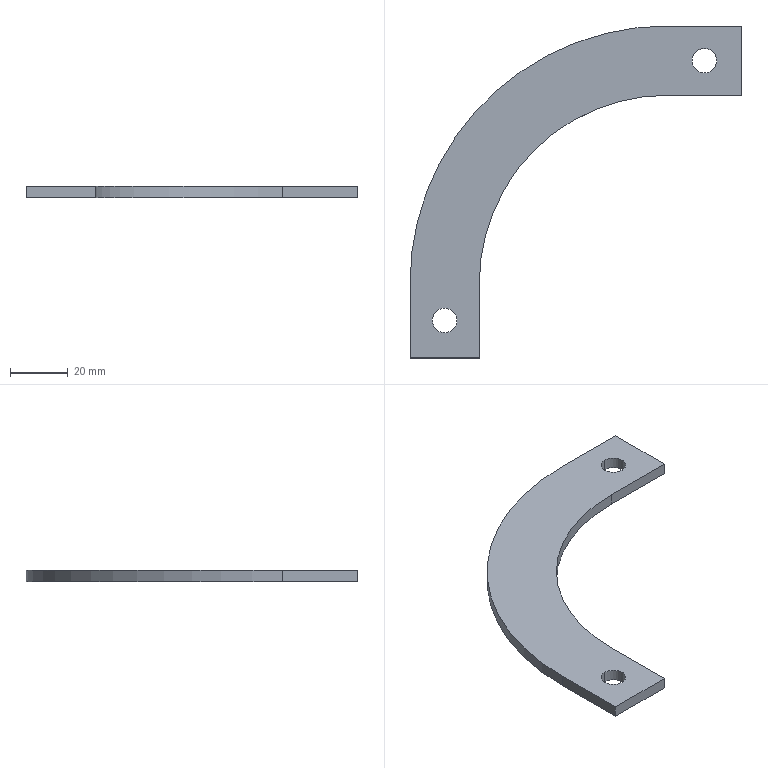Part | SolidWorks | features BaseBody 1 | 1 solid | 14 faces | box 115 x 115 x 4 mm | volume 16149 mm3 | plane 8 | cylinder 6 | commonest cylinder face diameters 8.5 x4 130 x1 178 x1
STEP:
#1=CARTESIAN_POINT('',(273.,59.25,281.));
#2=VERTEX_POINT('',#1);
#3=CARTESIAN_POINT('',(273.,50.75,281.));
#4=VERTEX_POINT('',#3);
#5=CARTESIAN_POINT('',(273.,55.,281.));
#6=DIRECTION('',(0.,0.,1.));
#7=DIRECTION('',(0.,1.,0.));
#8=AXIS2_PLACEMENT_3D('',#5,#6,#7);
#9=CIRCLE('',#8,4.25);
#10=EDGE_CURVE('',#2,#4,#9,.T.);
#11=ORIENTED_EDGE('',*,*,#10,.T.);
#12=CARTESIAN_POINT('',(273.,50.75,277.));
#13=VERTEX_POINT('',#12);
#14=CARTESIAN_POINT('',(273.,50.75,281.));
#15=DIRECTION('',(0.,0.,-1.));
#16=VECTOR('',#15,1000.);
#17=LINE('',#14,#16);
#18=EDGE_CURVE('',#4,#13,#17,.T.);
#19=ORIENTED_EDGE('',*,*,#18,.T.);
#20=CARTESIAN_POINT('',(273.,59.25,277.));
#21=VERTEX_POINT('',#20);
#22=CARTESIAN_POINT('',(273.,55.,277.));
#23=DIRECTION('',(0.,0.,-1.));
#24=DIRECTION('',(0.,-1.,0.));
#25=AXIS2_PLACEMENT_3D('',#22,#23,#24);
#26=CIRCLE('',#25,4.25);
#27=EDGE_CURVE('',#13,#21,#26,.T.);
#28=ORIENTED_EDGE('',*,*,#27,.T.);
#29=CARTESIAN_POINT('',(273.,59.25,281.));
#30=DIRECTION('',(0.,0.,-1.));
#31=VECTOR('',#30,1000.);
#32=LINE('',#29,#31);
#33=EDGE_CURVE('',#2,#21,#32,.T.);
#34=ORIENTED_EDGE('',*,*,#33,.F.);
#35=EDGE_LOOP('',(#11,#19,#28,#34));
#36=FACE_OUTER_BOUND('',#35,.T.);
#37=CARTESIAN_POINT('',(273.,55.,281.));
#38=DIRECTION('',(0.,0.,-1.));
#39=DIRECTION('',(0.,1.,0.));
#40=AXIS2_PLACEMENT_3D('',#37,#38,#39);
#41=CYLINDRICAL_SURFACE('',#40,4.25);
#42=ADVANCED_FACE('',(#36),#41,.F.);
#43=CARTESIAN_POINT('',(183.,-30.75,281.));
#44=VERTEX_POINT('',#43);
#45=CARTESIAN_POINT('',(183.,-39.25,281.));
#46=VERTEX_POINT('',#45);
#47=CARTESIAN_POINT('',(183.,-35.,281.));
#48=DIRECTION('',(0.,0.,1.));
#49=DIRECTION('',(0.,1.,0.));
#50=AXIS2_PLACEMENT_3D('',#47,#48,#49);
#51=CIRCLE('',#50,4.25);
#52=EDGE_CURVE('',#44,#46,#51,.T.);
#53=ORIENTED_EDGE('',*,*,#52,.T.);
#54=CARTESIAN_POINT('',(183.,-39.25,277.));
#55=VERTEX_POINT('',#54);
#56=CARTESIAN_POINT('',(183.,-39.25,281.));
#57=DIRECTION('',(0.,0.,-1.));
#58=VECTOR('',#57,1000.);
#59=LINE('',#56,#58);
#60=EDGE_CURVE('',#46,#55,#59,.T.);
#61=ORIENTED_EDGE('',*,*,#60,.T.);
#62=CARTESIAN_POINT('',(183.,-30.75,277.));
#63=VERTEX_POINT('',#62);
#64=CARTESIAN_POINT('',(183.,-35.,277.));
#65=DIRECTION('',(0.,0.,-1.));
#66=DIRECTION('',(0.,-1.,0.));
#67=AXIS2_PLACEMENT_3D('',#64,#65,#66);
#68=CIRCLE('',#67,4.25);
#69=EDGE_CURVE('',#55,#63,#68,.T.);
#70=ORIENTED_EDGE('',*,*,#69,.T.);
#71=CARTESIAN_POINT('',(183.,-30.75,281.));
#72=DIRECTION('',(0.,0.,-1.));
#73=VECTOR('',#72,1000.);
#74=LINE('',#71,#73);
#75=EDGE_CURVE('',#44,#63,#74,.T.);
#76=ORIENTED_EDGE('',*,*,#75,.F.);
#77=EDGE_LOOP('',(#53,#61,#70,#76));
#78=FACE_OUTER_BOUND('',#77,.T.);
#79=CARTESIAN_POINT('',(183.,-35.,281.));
#80=DIRECTION('',(0.,0.,-1.));
#81=DIRECTION('',(0.,1.,0.));
#82=AXIS2_PLACEMENT_3D('',#79,#80,#81);
#83=CYLINDRICAL_SURFACE('',#82,4.25);
#84=ADVANCED_FACE('',(#78),#83,.F.);
#85=CARTESIAN_POINT('',(183.,-35.,277.));
#86=DIRECTION('',(0.,0.,-1.));
#87=DIRECTION('',(0.,-1.,0.));
#88=AXIS2_PLACEMENT_3D('',#85,#86,#87);
#89=CIRCLE('',#88,4.25);
#90=EDGE_CURVE('',#63,#55,#89,.T.);
#91=ORIENTED_EDGE('',*,*,#90,.F.);
#92=ORIENTED_EDGE('',*,*,#69,.F.);
#93=EDGE_LOOP('',(#91,#92));
#94=FACE_BOUND('',#93,.T.);
#95=CARTESIAN_POINT('',(273.,55.,277.));
#96=DIRECTION('',(0.,0.,-1.));
#97=DIRECTION('',(0.,-1.,0.));
#98=AXIS2_PLACEMENT_3D('',#95,#96,#97);
#99=CIRCLE('',#98,4.25);
#100=EDGE_CURVE('',#21,#13,#99,.T.);
#101=ORIENTED_EDGE('',*,*,#100,.F.);
#102=ORIENTED_EDGE('',*,*,#27,.F.);
#103=EDGE_LOOP('',(#101,#102));
#104=FACE_BOUND('',#103,.T.);
#105=CARTESIAN_POINT('',(171.,-22.,277.));
#106=VERTEX_POINT('',#105);
#107=CARTESIAN_POINT('',(171.,-48.,277.));
#108=VERTEX_POINT('',#107);
#109=CARTESIAN_POINT('',(171.,-22.,277.));
#110=DIRECTION('',(0.,-1.,0.));
#111=VECTOR('',#110,1000.);
#112=LINE('',#109,#111);
#113=EDGE_CURVE('',#106,#108,#112,.T.);
#114=ORIENTED_EDGE('',*,*,#113,.F.);
#115=CARTESIAN_POINT('',(260.,67.,277.));
#116=VERTEX_POINT('',#115);
#117=CARTESIAN_POINT('',(260.,-22.,277.));
#118=DIRECTION('',(0.,0.,1.));
#119=DIRECTION('',(0.,1.,0.));
#120=AXIS2_PLACEMENT_3D('',#117,#118,#119);
#121=CIRCLE('',#120,89.);
#122=EDGE_CURVE('',#116,#106,#121,.T.);
#123=ORIENTED_EDGE('',*,*,#122,.F.);
#124=CARTESIAN_POINT('',(286.,67.,277.));
#125=VERTEX_POINT('',#124);
#126=CARTESIAN_POINT('',(286.,67.,277.));
#127=DIRECTION('',(-1.,0.,0.));
#128=VECTOR('',#127,1000.);
#129=LINE('',#126,#128);
#130=EDGE_CURVE('',#125,#116,#129,.T.);
#131=ORIENTED_EDGE('',*,*,#130,.F.);
#132=CARTESIAN_POINT('',(286.,43.,277.));
#133=VERTEX_POINT('',#132);
#134=CARTESIAN_POINT('',(286.,43.,277.));
#135=DIRECTION('',(0.,1.,0.));
#136=VECTOR('',#135,1000.);
#137=LINE('',#134,#136);
#138=EDGE_CURVE('',#133,#125,#137,.T.);
#139=ORIENTED_EDGE('',*,*,#138,.F.);
#140=CARTESIAN_POINT('',(260.,43.,277.));
#141=VERTEX_POINT('',#140);
#142=CARTESIAN_POINT('',(260.,43.,277.));
#143=DIRECTION('',(1.,0.,0.));
#144=VECTOR('',#143,1000.);
#145=LINE('',#142,#144);
#146=EDGE_CURVE('',#141,#133,#145,.T.);
#147=ORIENTED_EDGE('',*,*,#146,.F.);
#148=CARTESIAN_POINT('',(195.,-22.,277.));
#149=VERTEX_POINT('',#148);
#150=CARTESIAN_POINT('',(260.,-22.,277.));
#151=DIRECTION('',(0.,0.,-1.));
#152=DIRECTION('',(-1.,0.,0.));
#153=AXIS2_PLACEMENT_3D('',#150,#151,#152);
#154=CIRCLE('',#153,65.);
#155=EDGE_CURVE('',#149,#141,#154,.T.);
#156=ORIENTED_EDGE('',*,*,#155,.F.);
#157=CARTESIAN_POINT('',(195.,-48.,277.));
#158=VERTEX_POINT('',#157);
#159=CARTESIAN_POINT('',(195.,-48.,277.));
#160=DIRECTION('',(0.,1.,0.));
#161=VECTOR('',#160,1000.);
#162=LINE('',#159,#161);
#163=EDGE_CURVE('',#158,#149,#162,.T.);
#164=ORIENTED_EDGE('',*,*,#163,.F.);
#165=CARTESIAN_POINT('',(171.,-48.,277.));
#166=DIRECTION('',(1.,0.,0.));
#167=VECTOR('',#166,1000.);
#168=LINE('',#165,#167);
#169=EDGE_CURVE('',#108,#158,#168,.T.);
#170=ORIENTED_EDGE('',*,*,#169,.F.);
#171=EDGE_LOOP('',(#114,#123,#131,#139,#147,#156,#164,#170));
#172=FACE_OUTER_BOUND('',#171,.T.);
#173=CARTESIAN_POINT('',(260.,-22.,277.));
#174=DIRECTION('',(0.,0.,-1.));
#175=DIRECTION('',(-1.,0.,0.));
#176=AXIS2_PLACEMENT_3D('',#173,#174,#175);
#177=PLANE('',#176);
#178=ADVANCED_FACE('',(#94,#104,#172),#177,.T.);
#179=ORIENTED_EDGE('',*,*,#52,.F.);
#180=CARTESIAN_POINT('',(183.,-35.,281.));
#181=DIRECTION('',(0.,0.,1.));
#182=DIRECTION('',(0.,1.,0.));
#183=AXIS2_PLACEMENT_3D('',#180,#181,#182);
#184=CIRCLE('',#183,4.25);
#185=EDGE_CURVE('',#46,#44,#184,.T.);
#186=ORIENTED_EDGE('',*,*,#185,.F.);
#187=EDGE_LOOP('',(#179,#186));
#188=FACE_BOUND('',#187,.T.);
#189=ORIENTED_EDGE('',*,*,#10,.F.);
#190=CARTESIAN_POINT('',(273.,55.,281.));
#191=DIRECTION('',(0.,0.,1.));
#192=DIRECTION('',(0.,1.,0.));
#193=AXIS2_PLACEMENT_3D('',#190,#191,#192);
#194=CIRCLE('',#193,4.25);
#195=EDGE_CURVE('',#4,#2,#194,.T.);
#196=ORIENTED_EDGE('',*,*,#195,.F.);
#197=EDGE_LOOP('',(#189,#196));
#198=FACE_BOUND('',#197,.T.);
#199=CARTESIAN_POINT('',(171.,-48.,281.));
#200=VERTEX_POINT('',#199);
#201=CARTESIAN_POINT('',(171.,-22.,281.));
#202=VERTEX_POINT('',#201);
#203=CARTESIAN_POINT('',(171.,-48.,281.));
#204=DIRECTION('',(0.,1.,0.));
#205=VECTOR('',#204,1000.);
#206=LINE('',#203,#205);
#207=EDGE_CURVE('',#200,#202,#206,.T.);
#208=ORIENTED_EDGE('',*,*,#207,.F.);
#209=CARTESIAN_POINT('',(195.,-48.,281.));
#210=VERTEX_POINT('',#209);
#211=CARTESIAN_POINT('',(195.,-48.,281.));
#212=DIRECTION('',(-1.,0.,0.));
#213=VECTOR('',#212,1000.);
#214=LINE('',#211,#213);
#215=EDGE_CURVE('',#210,#200,#214,.T.);
#216=ORIENTED_EDGE('',*,*,#215,.F.);
#217=CARTESIAN_POINT('',(195.,-22.,281.));
#218=VERTEX_POINT('',#217);
#219=CARTESIAN_POINT('',(195.,-22.,281.));
#220=DIRECTION('',(0.,-1.,0.));
#221=VECTOR('',#220,1000.);
#222=LINE('',#219,#221);
#223=EDGE_CURVE('',#218,#210,#222,.T.);
#224=ORIENTED_EDGE('',*,*,#223,.F.);
#225=CARTESIAN_POINT('',(260.,43.,281.));
#226=VERTEX_POINT('',#225);
#227=CARTESIAN_POINT('',(260.,-22.,281.));
#228=DIRECTION('',(0.,0.,1.));
#229=DIRECTION('',(0.,1.,0.));
#230=AXIS2_PLACEMENT_3D('',#227,#228,#229);
#231=CIRCLE('',#230,65.);
#232=EDGE_CURVE('',#226,#218,#231,.T.);
#233=ORIENTED_EDGE('',*,*,#232,.F.);
#234=CARTESIAN_POINT('',(286.,43.,281.));
#235=VERTEX_POINT('',#234);
#236=CARTESIAN_POINT('',(286.,43.,281.));
#237=DIRECTION('',(-1.,0.,0.));
#238=VECTOR('',#237,1000.);
#239=LINE('',#236,#238);
#240=EDGE_CURVE('',#235,#226,#239,.T.);
#241=ORIENTED_EDGE('',*,*,#240,.F.);
#242=CARTESIAN_POINT('',(286.,67.,281.));
#243=VERTEX_POINT('',#242);
#244=CARTESIAN_POINT('',(286.,67.,281.));
#245=DIRECTION('',(0.,-1.,0.));
#246=VECTOR('',#245,1000.);
#247=LINE('',#244,#246);
#248=EDGE_CURVE('',#243,#235,#247,.T.);
#249=ORIENTED_EDGE('',*,*,#248,.F.);
#250=CARTESIAN_POINT('',(260.,67.,281.));
#251=VERTEX_POINT('',#250);
#252=CARTESIAN_POINT('',(260.,67.,281.));
#253=DIRECTION('',(1.,0.,0.));
#254=VECTOR('',#253,1000.);
#255=LINE('',#252,#254);
#256=EDGE_CURVE('',#251,#243,#255,.T.);
#257=ORIENTED_EDGE('',*,*,#256,.F.);
#258=CARTESIAN_POINT('',(260.,-22.,281.));
#259=DIRECTION('',(0.,0.,-1.));
#260=DIRECTION('',(-1.,0.,0.));
#261=AXIS2_PLACEMENT_3D('',#258,#259,#260);
#262=CIRCLE('',#261,89.);
#263=EDGE_CURVE('',#202,#251,#262,.T.);
#264=ORIENTED_EDGE('',*,*,#263,.F.);
#265=EDGE_LOOP('',(#208,#216,#224,#233,#241,#249,#257,#264));
#266=FACE_OUTER_BOUND('',#265,.T.);
#267=CARTESIAN_POINT('',(260.,-22.,281.));
#268=DIRECTION('',(0.,0.,1.));
#269=DIRECTION('',(0.,-1.,0.));
#270=AXIS2_PLACEMENT_3D('',#267,#268,#269);
#271=PLANE('',#270);
#272=ADVANCED_FACE('',(#188,#198,#266),#271,.T.);
#273=ORIENTED_EDGE('',*,*,#60,.F.);
#274=ORIENTED_EDGE('',*,*,#185,.T.);
#275=ORIENTED_EDGE('',*,*,#75,.T.);
#276=ORIENTED_EDGE('',*,*,#90,.T.);
#277=EDGE_LOOP('',(#273,#274,#275,#276));
#278=FACE_OUTER_BOUND('',#277,.T.);
#279=CARTESIAN_POINT('',(183.,-35.,281.));
#280=DIRECTION('',(0.,0.,-1.));
#281=DIRECTION('',(0.,1.,0.));
#282=AXIS2_PLACEMENT_3D('',#279,#280,#281);
#283=CYLINDRICAL_SURFACE('',#282,4.25);
#284=ADVANCED_FACE('',(#278),#283,.F.);
#285=ORIENTED_EDGE('',*,*,#169,.T.);
#286=CARTESIAN_POINT('',(195.,-48.,281.));
#287=DIRECTION('',(0.,0.,-1.));
#288=VECTOR('',#287,1000.);
#289=LINE('',#286,#288);
#290=EDGE_CURVE('',#210,#158,#289,.T.);
#291=ORIENTED_EDGE('',*,*,#290,.F.);
#292=ORIENTED_EDGE('',*,*,#215,.T.);
#293=CARTESIAN_POINT('',(171.,-48.,277.));
#294=DIRECTION('',(0.,0.,1.));
#295=VECTOR('',#294,1000.);
#296=LINE('',#293,#295);
#297=EDGE_CURVE('',#108,#200,#296,.T.);
#298=ORIENTED_EDGE('',*,*,#297,.F.);
#299=EDGE_LOOP('',(#285,#291,#292,#298));
#300=FACE_OUTER_BOUND('',#299,.T.);
#301=CARTESIAN_POINT('',(195.,-48.,281.));
#302=DIRECTION('',(0.,-1.,0.));
#303=DIRECTION('',(0.,0.,-1.));
#304=AXIS2_PLACEMENT_3D('',#301,#302,#303);
#305=PLANE('',#304);
#306=ADVANCED_FACE('',(#300),#305,.T.);
#307=ORIENTED_EDGE('',*,*,#18,.F.);
#308=ORIENTED_EDGE('',*,*,#195,.T.);
#309=ORIENTED_EDGE('',*,*,#33,.T.);
#310=ORIENTED_EDGE('',*,*,#100,.T.);
#311=EDGE_LOOP('',(#307,#308,#309,#310));
#312=FACE_OUTER_BOUND('',#311,.T.);
#313=CARTESIAN_POINT('',(273.,55.,281.));
#314=DIRECTION('',(0.,0.,-1.));
#315=DIRECTION('',(0.,1.,0.));
#316=AXIS2_PLACEMENT_3D('',#313,#314,#315);
#317=CYLINDRICAL_SURFACE('',#316,4.25);
#318=ADVANCED_FACE('',(#312),#317,.F.);
#319=ORIENTED_EDGE('',*,*,#163,.T.);
#320=CARTESIAN_POINT('',(195.,-22.,281.));
#321=DIRECTION('',(0.,0.,-1.));
#322=VECTOR('',#321,1000.);
#323=LINE('',#320,#322);
#324=EDGE_CURVE('',#218,#149,#323,.T.);
#325=ORIENTED_EDGE('',*,*,#324,.F.);
#326=ORIENTED_EDGE('',*,*,#223,.T.);
#327=ORIENTED_EDGE('',*,*,#290,.T.);
#328=EDGE_LOOP('',(#319,#325,#326,#327));
#329=FACE_OUTER_BOUND('',#328,.T.);
#330=CARTESIAN_POINT('',(195.,-22.,281.));
#331=DIRECTION('',(1.,0.,0.));
#332=DIRECTION('',(0.,-1.,0.));
#333=AXIS2_PLACEMENT_3D('',#330,#331,#332);
#334=PLANE('',#333);
#335=ADVANCED_FACE('',(#329),#334,.T.);
#336=ORIENTED_EDGE('',*,*,#155,.T.);
#337=CARTESIAN_POINT('',(260.,43.,281.));
#338=DIRECTION('',(0.,0.,-1.));
#339=VECTOR('',#338,1000.);
#340=LINE('',#337,#339);
#341=EDGE_CURVE('',#226,#141,#340,.T.);
#342=ORIENTED_EDGE('',*,*,#341,.F.);
#343=ORIENTED_EDGE('',*,*,#232,.T.);
#344=ORIENTED_EDGE('',*,*,#324,.T.);
#345=EDGE_LOOP('',(#336,#342,#343,#344));
#346=FACE_OUTER_BOUND('',#345,.T.);
#347=CARTESIAN_POINT('',(260.,-22.,281.));
#348=DIRECTION('',(0.,0.,-1.));
#349=DIRECTION('',(1.,0.,0.));
#350=AXIS2_PLACEMENT_3D('',#347,#348,#349);
#351=CYLINDRICAL_SURFACE('',#350,65.);
#352=ADVANCED_FACE('',(#346),#351,.F.);
#353=ORIENTED_EDGE('',*,*,#146,.T.);
#354=CARTESIAN_POINT('',(286.,43.,281.));
#355=DIRECTION('',(0.,0.,-1.));
#356=VECTOR('',#355,1000.);
#357=LINE('',#354,#356);
#358=EDGE_CURVE('',#235,#133,#357,.T.);
#359=ORIENTED_EDGE('',*,*,#358,.F.);
#360=ORIENTED_EDGE('',*,*,#240,.T.);
#361=ORIENTED_EDGE('',*,*,#341,.T.);
#362=EDGE_LOOP('',(#353,#359,#360,#361));
#363=FACE_OUTER_BOUND('',#362,.T.);
#364=CARTESIAN_POINT('',(286.,43.,281.));
#365=DIRECTION('',(0.,-1.,0.));
#366=DIRECTION('',(0.,0.,-1.));
#367=AXIS2_PLACEMENT_3D('',#364,#365,#366);
#368=PLANE('',#367);
#369=ADVANCED_FACE('',(#363),#368,.T.);
#370=ORIENTED_EDGE('',*,*,#138,.T.);
#371=CARTESIAN_POINT('',(286.,67.,281.));
#372=DIRECTION('',(0.,0.,-1.));
#373=VECTOR('',#372,1000.);
#374=LINE('',#371,#373);
#375=EDGE_CURVE('',#243,#125,#374,.T.);
#376=ORIENTED_EDGE('',*,*,#375,.F.);
#377=ORIENTED_EDGE('',*,*,#248,.T.);
#378=ORIENTED_EDGE('',*,*,#358,.T.);
#379=EDGE_LOOP('',(#370,#376,#377,#378));
#380=FACE_OUTER_BOUND('',#379,.T.);
#381=CARTESIAN_POINT('',(286.,67.,281.));
#382=DIRECTION('',(1.,0.,0.));
#383=DIRECTION('',(0.,-1.,0.));
#384=AXIS2_PLACEMENT_3D('',#381,#382,#383);
#385=PLANE('',#384);
#386=ADVANCED_FACE('',(#380),#385,.T.);
#387=ORIENTED_EDGE('',*,*,#130,.T.);
#388=CARTESIAN_POINT('',(260.,67.,281.));
#389=DIRECTION('',(0.,0.,-1.));
#390=VECTOR('',#389,1000.);
#391=LINE('',#388,#390);
#392=EDGE_CURVE('',#251,#116,#391,.T.);
#393=ORIENTED_EDGE('',*,*,#392,.F.);
#394=ORIENTED_EDGE('',*,*,#256,.T.);
#395=ORIENTED_EDGE('',*,*,#375,.T.);
#396=EDGE_LOOP('',(#387,#393,#394,#395));
#397=FACE_OUTER_BOUND('',#396,.T.);
#398=CARTESIAN_POINT('',(260.,67.,281.));
#399=DIRECTION('',(0.,1.,0.));
#400=DIRECTION('',(0.,0.,-1.));
#401=AXIS2_PLACEMENT_3D('',#398,#399,#400);
#402=PLANE('',#401);
#403=ADVANCED_FACE('',(#397),#402,.T.);
#404=ORIENTED_EDGE('',*,*,#122,.T.);
#405=CARTESIAN_POINT('',(171.,-22.,281.));
#406=DIRECTION('',(0.,0.,-1.));
#407=VECTOR('',#406,1000.);
#408=LINE('',#405,#407);
#409=EDGE_CURVE('',#202,#106,#408,.T.);
#410=ORIENTED_EDGE('',*,*,#409,.F.);
#411=ORIENTED_EDGE('',*,*,#263,.T.);
#412=ORIENTED_EDGE('',*,*,#392,.T.);
#413=EDGE_LOOP('',(#404,#410,#411,#412));
#414=FACE_OUTER_BOUND('',#413,.T.);
#415=CARTESIAN_POINT('',(260.,-22.,281.));
#416=DIRECTION('',(0.,0.,-1.));
#417=DIRECTION('',(0.,-1.,0.));
#418=AXIS2_PLACEMENT_3D('',#415,#416,#417);
#419=CYLINDRICAL_SURFACE('',#418,89.);
#420=ADVANCED_FACE('',(#414),#419,.T.);
#421=ORIENTED_EDGE('',*,*,#113,.T.);
#422=ORIENTED_EDGE('',*,*,#297,.T.);
#423=ORIENTED_EDGE('',*,*,#207,.T.);
#424=ORIENTED_EDGE('',*,*,#409,.T.);
#425=EDGE_LOOP('',(#421,#422,#423,#424));
#426=FACE_OUTER_BOUND('',#425,.T.);
#427=CARTESIAN_POINT('',(171.,-48.,281.));
#428=DIRECTION('',(-1.,0.,0.));
#429=DIRECTION('',(0.,0.,1.));
#430=AXIS2_PLACEMENT_3D('',#427,#428,#429);
#431=PLANE('',#430);
#432=ADVANCED_FACE('',(#426),#431,.T.);
#433=CLOSED_SHELL('',(#42,#84,#178,#272,#284,#306,#318,#335,#352,#369,#386,#403,#420,#432));
#434=MANIFOLD_SOLID_BREP('',#433);
#435=CARTESIAN_POINT('',(0.,0.,0.));
#436=DIRECTION('',(0.,0.,1.));
#437=DIRECTION('',(1.,0.,0.));
#438=AXIS2_PLACEMENT_3D('',#435,#436,#437);
#439=(LENGTH_UNIT()NAMED_UNIT(*)SI_UNIT(.MILLI.,.METRE.));
#440=UNCERTAINTY_MEASURE_WITH_UNIT(LENGTH_MEASURE(0.00001),#439,'','');
#441=(NAMED_UNIT(*)PLANE_ANGLE_UNIT()SI_UNIT($,.RADIAN.));
#442=(NAMED_UNIT(*)SI_UNIT($,.STERADIAN.)SOLID_ANGLE_UNIT());
#443=(GEOMETRIC_REPRESENTATION_CONTEXT(3)GLOBAL_UNCERTAINTY_ASSIGNED_CONTEXT((#440))GLOBAL_UNIT_ASSIGNED_CONTEXT((#439,#441,#442))REPRESENTATION_CONTEXT('',''));
#444=ADVANCED_BREP_SHAPE_REPRESENTATION('',(#434,#438),#443);